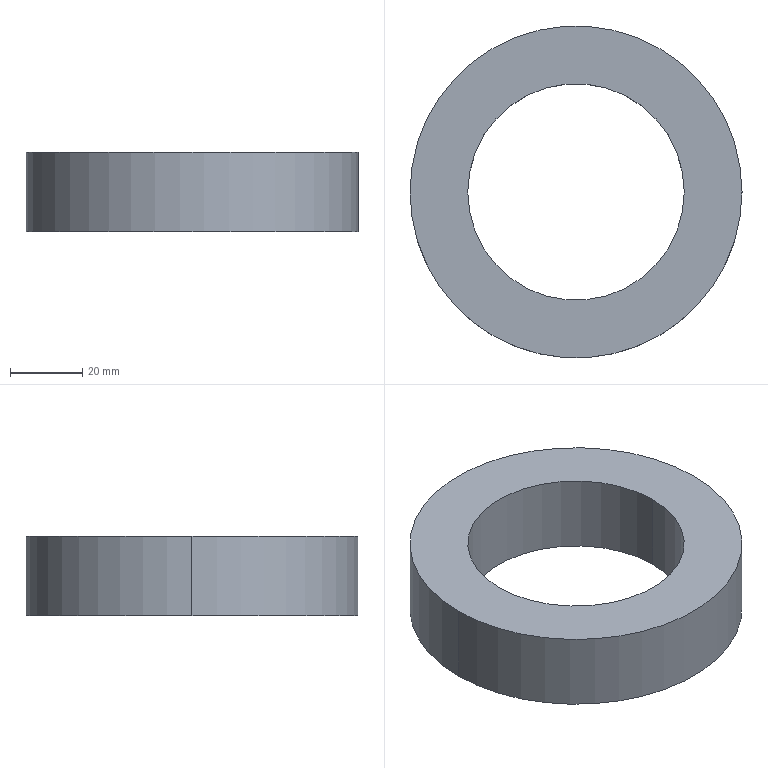Part | SolidWorks | features Extrusion 1 | 1 solid | 6 faces | box 92 x 92 x 22 mm | volume 84044 mm3 | cylinder 4 | plane 2 | commonest cylinder face diameters 60 x2 92 x2
STEP:
#1=CARTESIAN_POINT('',(-30.,0.,22.));
#2=VERTEX_POINT('',#1);
#3=CARTESIAN_POINT('',(30.,0.,22.));
#4=VERTEX_POINT('',#3);
#5=CARTESIAN_POINT('',(0.,0.,22.));
#6=DIRECTION('',(0.,0.,1.));
#7=DIRECTION('',(1.,0.,0.));
#8=AXIS2_PLACEMENT_3D('',#5,#6,#7);
#9=CIRCLE('',#8,30.);
#10=EDGE_CURVE('',#2,#4,#9,.T.);
#11=ORIENTED_EDGE('',*,*,#10,.T.);
#12=CARTESIAN_POINT('',(30.,0.,0.));
#13=VERTEX_POINT('',#12);
#14=CARTESIAN_POINT('',(30.,0.,22.));
#15=DIRECTION('',(0.,0.,-1.));
#16=VECTOR('',#15,1000.);
#17=LINE('',#14,#16);
#18=EDGE_CURVE('',#4,#13,#17,.T.);
#19=ORIENTED_EDGE('',*,*,#18,.T.);
#20=CARTESIAN_POINT('',(-30.,0.,0.));
#21=VERTEX_POINT('',#20);
#22=CARTESIAN_POINT('',(0.,0.,0.));
#23=DIRECTION('',(0.,0.,1.));
#24=DIRECTION('',(1.,0.,0.));
#25=AXIS2_PLACEMENT_3D('',#22,#23,#24);
#26=CIRCLE('',#25,30.);
#27=EDGE_CURVE('',#21,#13,#26,.T.);
#28=ORIENTED_EDGE('',*,*,#27,.F.);
#29=CARTESIAN_POINT('',(-30.,0.,22.));
#30=DIRECTION('',(0.,0.,-1.));
#31=VECTOR('',#30,1000.);
#32=LINE('',#29,#31);
#33=EDGE_CURVE('',#2,#21,#32,.T.);
#34=ORIENTED_EDGE('',*,*,#33,.F.);
#35=EDGE_LOOP('',(#11,#19,#28,#34));
#36=FACE_OUTER_BOUND('',#35,.T.);
#37=CARTESIAN_POINT('',(0.,0.,22.));
#38=DIRECTION('',(0.,0.,-1.));
#39=DIRECTION('',(-1.,0.,0.));
#40=AXIS2_PLACEMENT_3D('',#37,#38,#39);
#41=CYLINDRICAL_SURFACE('',#40,30.);
#42=ADVANCED_FACE('',(#36),#41,.F.);
#43=CARTESIAN_POINT('',(46.,0.,22.));
#44=VERTEX_POINT('',#43);
#45=CARTESIAN_POINT('',(-46.,0.,22.));
#46=VERTEX_POINT('',#45);
#47=CARTESIAN_POINT('',(0.,0.,22.));
#48=DIRECTION('',(0.,0.,1.));
#49=DIRECTION('',(1.,0.,0.));
#50=AXIS2_PLACEMENT_3D('',#47,#48,#49);
#51=CIRCLE('',#50,46.);
#52=EDGE_CURVE('',#44,#46,#51,.T.);
#53=ORIENTED_EDGE('',*,*,#52,.F.);
#54=CARTESIAN_POINT('',(46.,0.,0.));
#55=VERTEX_POINT('',#54);
#56=CARTESIAN_POINT('',(46.,0.,22.));
#57=DIRECTION('',(0.,0.,-1.));
#58=VECTOR('',#57,1000.);
#59=LINE('',#56,#58);
#60=EDGE_CURVE('',#44,#55,#59,.T.);
#61=ORIENTED_EDGE('',*,*,#60,.T.);
#62=CARTESIAN_POINT('',(-46.,0.,0.));
#63=VERTEX_POINT('',#62);
#64=CARTESIAN_POINT('',(0.,0.,0.));
#65=DIRECTION('',(0.,0.,1.));
#66=DIRECTION('',(1.,0.,0.));
#67=AXIS2_PLACEMENT_3D('',#64,#65,#66);
#68=CIRCLE('',#67,46.);
#69=EDGE_CURVE('',#55,#63,#68,.T.);
#70=ORIENTED_EDGE('',*,*,#69,.T.);
#71=CARTESIAN_POINT('',(-46.,0.,22.));
#72=DIRECTION('',(0.,0.,-1.));
#73=VECTOR('',#72,1000.);
#74=LINE('',#71,#73);
#75=EDGE_CURVE('',#46,#63,#74,.T.);
#76=ORIENTED_EDGE('',*,*,#75,.F.);
#77=EDGE_LOOP('',(#53,#61,#70,#76));
#78=FACE_OUTER_BOUND('',#77,.T.);
#79=CARTESIAN_POINT('',(0.,0.,22.));
#80=DIRECTION('',(0.,0.,-1.));
#81=DIRECTION('',(-1.,0.,0.));
#82=AXIS2_PLACEMENT_3D('',#79,#80,#81);
#83=CYLINDRICAL_SURFACE('',#82,46.);
#84=ADVANCED_FACE('',(#78),#83,.T.);
#85=CARTESIAN_POINT('',(0.,0.,22.));
#86=DIRECTION('',(0.,0.,1.));
#87=DIRECTION('',(1.,0.,0.));
#88=AXIS2_PLACEMENT_3D('',#85,#86,#87);
#89=CIRCLE('',#88,46.);
#90=EDGE_CURVE('',#46,#44,#89,.T.);
#91=ORIENTED_EDGE('',*,*,#90,.T.);
#92=ORIENTED_EDGE('',*,*,#52,.T.);
#93=EDGE_LOOP('',(#91,#92));
#94=FACE_OUTER_BOUND('',#93,.T.);
#95=ORIENTED_EDGE('',*,*,#10,.F.);
#96=CARTESIAN_POINT('',(0.,0.,22.));
#97=DIRECTION('',(0.,0.,1.));
#98=DIRECTION('',(1.,0.,0.));
#99=AXIS2_PLACEMENT_3D('',#96,#97,#98);
#100=CIRCLE('',#99,30.);
#101=EDGE_CURVE('',#4,#2,#100,.T.);
#102=ORIENTED_EDGE('',*,*,#101,.F.);
#103=EDGE_LOOP('',(#95,#102));
#104=FACE_BOUND('',#103,.T.);
#105=CARTESIAN_POINT('',(0.,0.,22.));
#106=DIRECTION('',(0.,0.,1.));
#107=DIRECTION('',(1.,0.,0.));
#108=AXIS2_PLACEMENT_3D('',#105,#106,#107);
#109=PLANE('',#108);
#110=ADVANCED_FACE('',(#94,#104),#109,.T.);
#111=CARTESIAN_POINT('',(0.,0.,0.));
#112=DIRECTION('',(0.,0.,1.));
#113=DIRECTION('',(1.,0.,0.));
#114=AXIS2_PLACEMENT_3D('',#111,#112,#113);
#115=CIRCLE('',#114,46.);
#116=EDGE_CURVE('',#63,#55,#115,.T.);
#117=ORIENTED_EDGE('',*,*,#116,.F.);
#118=ORIENTED_EDGE('',*,*,#69,.F.);
#119=EDGE_LOOP('',(#117,#118));
#120=FACE_OUTER_BOUND('',#119,.T.);
#121=ORIENTED_EDGE('',*,*,#27,.T.);
#122=CARTESIAN_POINT('',(0.,0.,0.));
#123=DIRECTION('',(0.,0.,1.));
#124=DIRECTION('',(1.,0.,0.));
#125=AXIS2_PLACEMENT_3D('',#122,#123,#124);
#126=CIRCLE('',#125,30.);
#127=EDGE_CURVE('',#13,#21,#126,.T.);
#128=ORIENTED_EDGE('',*,*,#127,.T.);
#129=EDGE_LOOP('',(#121,#128));
#130=FACE_BOUND('',#129,.T.);
#131=CARTESIAN_POINT('',(0.,0.,0.));
#132=DIRECTION('',(0.,0.,1.));
#133=DIRECTION('',(1.,0.,0.));
#134=AXIS2_PLACEMENT_3D('',#131,#132,#133);
#135=PLANE('',#134);
#136=ADVANCED_FACE('',(#120,#130),#135,.F.);
#137=ORIENTED_EDGE('',*,*,#60,.F.);
#138=ORIENTED_EDGE('',*,*,#90,.F.);
#139=ORIENTED_EDGE('',*,*,#75,.T.);
#140=ORIENTED_EDGE('',*,*,#116,.T.);
#141=EDGE_LOOP('',(#137,#138,#139,#140));
#142=FACE_OUTER_BOUND('',#141,.T.);
#143=CARTESIAN_POINT('',(0.,0.,22.));
#144=DIRECTION('',(0.,0.,-1.));
#145=DIRECTION('',(-1.,0.,0.));
#146=AXIS2_PLACEMENT_3D('',#143,#144,#145);
#147=CYLINDRICAL_SURFACE('',#146,46.);
#148=ADVANCED_FACE('',(#142),#147,.T.);
#149=ORIENTED_EDGE('',*,*,#18,.F.);
#150=ORIENTED_EDGE('',*,*,#101,.T.);
#151=ORIENTED_EDGE('',*,*,#33,.T.);
#152=ORIENTED_EDGE('',*,*,#127,.F.);
#153=EDGE_LOOP('',(#149,#150,#151,#152));
#154=FACE_OUTER_BOUND('',#153,.T.);
#155=CARTESIAN_POINT('',(0.,0.,22.));
#156=DIRECTION('',(0.,0.,-1.));
#157=DIRECTION('',(-1.,0.,0.));
#158=AXIS2_PLACEMENT_3D('',#155,#156,#157);
#159=CYLINDRICAL_SURFACE('',#158,30.);
#160=ADVANCED_FACE('',(#154),#159,.F.);
#161=CLOSED_SHELL('',(#42,#84,#110,#136,#148,#160));
#162=MANIFOLD_SOLID_BREP('',#161);
#163=CARTESIAN_POINT('',(0.,0.,0.));
#164=DIRECTION('',(0.,0.,1.));
#165=DIRECTION('',(1.,0.,0.));
#166=AXIS2_PLACEMENT_3D('',#163,#164,#165);
#167=(LENGTH_UNIT()NAMED_UNIT(*)SI_UNIT(.MILLI.,.METRE.));
#168=UNCERTAINTY_MEASURE_WITH_UNIT(LENGTH_MEASURE(0.00001),#167,'','');
#169=(NAMED_UNIT(*)PLANE_ANGLE_UNIT()SI_UNIT($,.RADIAN.));
#170=(NAMED_UNIT(*)SI_UNIT($,.STERADIAN.)SOLID_ANGLE_UNIT());
#171=(GEOMETRIC_REPRESENTATION_CONTEXT(3)GLOBAL_UNCERTAINTY_ASSIGNED_CONTEXT((#168))GLOBAL_UNIT_ASSIGNED_CONTEXT((#167,#169,#170))REPRESENTATION_CONTEXT('',''));
#172=ADVANCED_BREP_SHAPE_REPRESENTATION('',(#162,#166),#171);